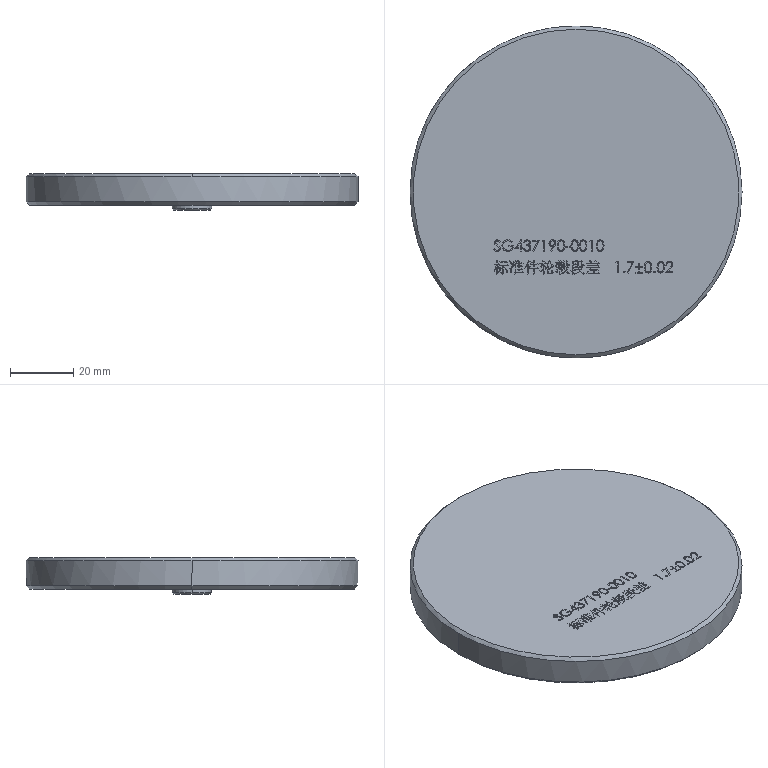Part | STEP file | Mkt hub std part | 1 solid | 695 faces | box 105 x 105 x 11.7 mm | volume 77844 mm3 | plane 455 | spline 226 | cone 8 | cylinder 6 | commonest cylinder face diameters 12.5 x2 75 x2 105 x2